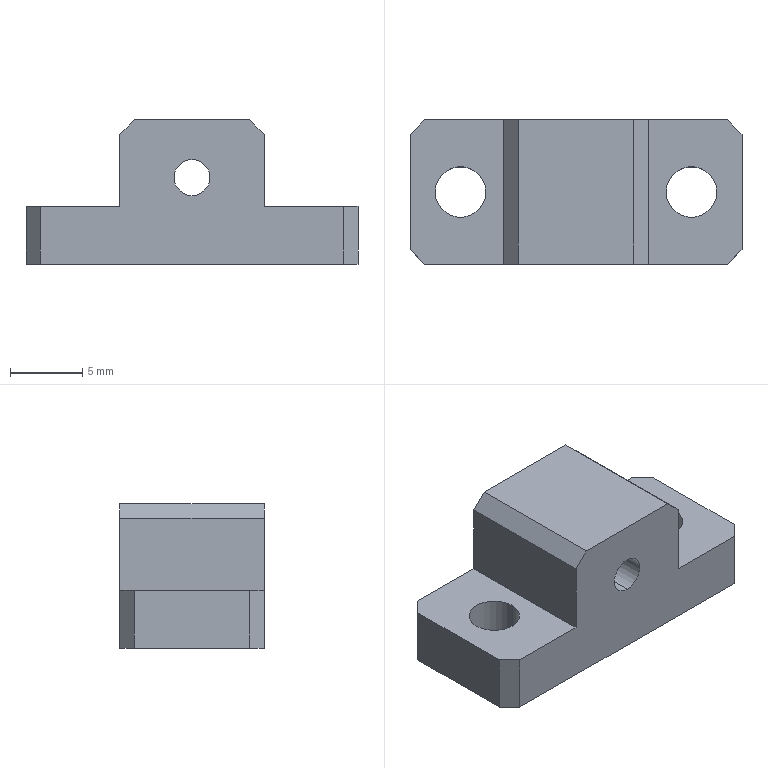Part | STEP file | PN_0031 Mount electronic clip fiber sensor seat B | 1 solid | 22 faces | box 23 x 10 x 10 mm | volume 1376 mm3 | plane 16 | cylinder 6 | commonest cylinder face diameters 3.5 x4 2.5 x2